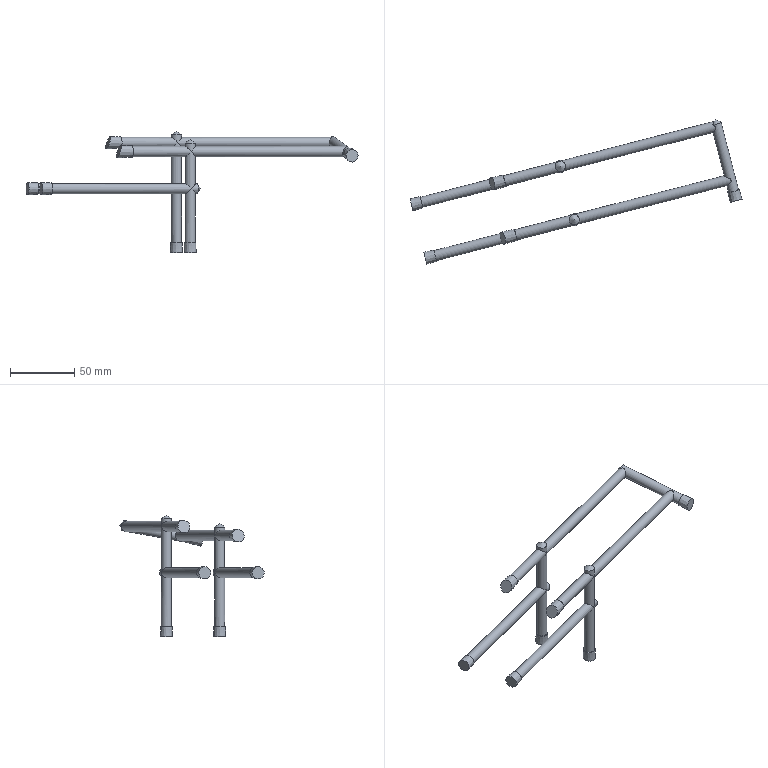Part | STEP file | 车灯-后视镜_id398_x_t | 1 solid | 43 faces | box 259.149 x 112.453 x 94.778 mm | volume 42702 mm3 | cylinder 15 | plane 14 | cone 14 | commonest cylinder face diameters 8 x15
STEP:
#1=CARTESIAN_POINT('',(-127.487,12.001,14.714));
#2=VERTEX_POINT('',#1);
#3=CARTESIAN_POINT('',(-129.485,19.747,14.714));
#4=VERTEX_POINT('',#3);
#5=CARTESIAN_POINT('',(-128.486,15.874,14.714));
#6=DIRECTION('',(-0.6847,-0.1766,-0.7071));
#7=DIRECTION('',(-0.6847,-0.1766,0.7071));
#8=AXIS2_PLACEMENT_3D('',#5,#6,#7);
#9=ELLIPSE('',#8,5.657,4.);
#10=EDGE_CURVE('',#2,#4,#9,.T.);
#11=ORIENTED_EDGE('',*,*,#10,.F.);
#12=CARTESIAN_POINT('',(-128.486,15.874,14.714));
#13=DIRECTION('',(0.6847,0.1766,-0.7071));
#14=DIRECTION('',(0.6847,0.1766,0.7071));
#15=AXIS2_PLACEMENT_3D('',#12,#13,#14);
#16=ELLIPSE('',#15,5.657,4.);
#17=EDGE_CURVE('',#4,#2,#16,.T.);
#18=ORIENTED_EDGE('',*,*,#17,.F.);
#19=EDGE_LOOP('',(#11,#18));
#20=FACE_BOUND('',#19,.T.);
#21=CARTESIAN_POINT('',(-127.487,12.001,43.714));
#22=VERTEX_POINT('',#21);
#23=CARTESIAN_POINT('',(-129.485,19.747,43.714));
#24=VERTEX_POINT('',#23);
#25=CARTESIAN_POINT('',(-128.486,15.874,43.714));
#26=DIRECTION('',(0.6847,0.1766,-0.7071));
#27=DIRECTION('',(0.6847,0.1766,0.7071));
#28=AXIS2_PLACEMENT_3D('',#25,#26,#27);
#29=ELLIPSE('',#28,5.657,4.);
#30=EDGE_CURVE('',#22,#24,#29,.T.);
#31=ORIENTED_EDGE('',*,*,#30,.T.);
#32=CARTESIAN_POINT('',(-128.486,15.874,43.714));
#33=DIRECTION('',(-0.6847,-0.1766,-0.7071));
#34=DIRECTION('',(0.6847,0.1766,-0.7071));
#35=AXIS2_PLACEMENT_3D('',#32,#33,#34);
#36=ELLIPSE('',#35,5.657,4.);
#37=EDGE_CURVE('',#24,#22,#36,.T.);
#38=ORIENTED_EDGE('',*,*,#37,.T.);
#39=EDGE_LOOP('',(#31,#38));
#40=FACE_BOUND('',#39,.T.);
#41=CARTESIAN_POINT('',(-128.486,15.874,-34.206));
#42=DIRECTION('',(0.,0.,1.));
#43=DIRECTION('',(-0.9683,-0.2497,0.));
#44=AXIS2_PLACEMENT_3D('',#41,#42,#43);
#45=CYLINDRICAL_SURFACE('',#44,4.);
#46=ADVANCED_FACE('',(#20,#40),#45,.T.);
#47=ORIENTED_EDGE('',*,*,#37,.F.);
#48=CARTESIAN_POINT('',(-128.486,15.874,43.714));
#49=DIRECTION('',(-0.6847,-0.1766,0.7071));
#50=DIRECTION('',(0.6847,0.1766,0.7071));
#51=AXIS2_PLACEMENT_3D('',#48,#49,#50);
#52=ELLIPSE('',#51,5.657,4.);
#53=EDGE_CURVE('',#22,#24,#52,.T.);
#54=ORIENTED_EDGE('',*,*,#53,.F.);
#55=EDGE_LOOP('',(#47,#54));
#56=FACE_BOUND('',#55,.T.);
#57=CARTESIAN_POINT('',(-6.607,48.159,47.628));
#58=VERTEX_POINT('',#57);
#59=CARTESIAN_POINT('',(-5.871,45.306,47.108));
#60=VERTEX_POINT('',#59);
#61=CARTESIAN_POINT('',(-6.4,47.356,43.714));
#62=DIRECTION('',(0.9683,0.2497,0.));
#63=DIRECTION('',(0.,0.,-1.));
#64=AXIS2_PLACEMENT_3D('',#61,#62,#63);
#65=CIRCLE('',#64,4.);
#66=EDGE_CURVE('',#58,#60,#65,.T.);
#67=ORIENTED_EDGE('',*,*,#66,.F.);
#68=CARTESIAN_POINT('',(-6.607,48.159,47.628));
#69=CARTESIAN_POINT('',(-7.16,48.016,47.628));
#70=CARTESIAN_POINT('',(-7.723,48.193,47.564));
#71=CARTESIAN_POINT('',(-8.745,48.599,47.309));
#72=CARTESIAN_POINT('',(-9.21,48.843,47.121));
#73=CARTESIAN_POINT('',(-10.495,49.569,46.31));
#74=CARTESIAN_POINT('',(-11.18,50.053,45.377));
#75=CARTESIAN_POINT('',(-11.339,50.334,43.164));
#76=CARTESIAN_POINT('',(-10.794,50.106,42.047));
#77=CARTESIAN_POINT('',(-9.74,49.476,40.904));
#78=CARTESIAN_POINT('',(-9.342,49.219,40.587));
#79=CARTESIAN_POINT('',(-8.57,48.586,40.078));
#80=CARTESIAN_POINT('',(-8.159,48.193,39.872));
#81=CARTESIAN_POINT('',(-7.882,47.108,39.676));
#82=CARTESIAN_POINT('',(-8.042,46.529,39.705));
#83=CARTESIAN_POINT('',(-8.382,45.48,39.909));
#84=CARTESIAN_POINT('',(-8.581,44.986,40.086));
#85=CARTESIAN_POINT('',(-9.117,43.59,40.865));
#86=CARTESIAN_POINT('',(-9.391,42.791,41.774));
#87=CARTESIAN_POINT('',(-9.197,42.352,43.97));
#88=CARTESIAN_POINT('',(-8.744,42.76,45.063));
#89=CARTESIAN_POINT('',(-7.887,43.686,46.177));
#90=CARTESIAN_POINT('',(-7.573,44.046,46.479));
#91=CARTESIAN_POINT('',(-6.845,44.772,46.94));
#92=CARTESIAN_POINT('',(-6.422,45.164,47.108));
#93=CARTESIAN_POINT('',(-5.871,45.306,47.108));
#94=B_SPLINE_CURVE_WITH_KNOTS('',3,(#68,#69,#70,#71,#72,#73,#74,#75,#76,#77,#78,#79,#80,#81,#82,#83,#84,#85,#86,#87,#88,#89,#90,#91,#92,#93),.UNSPECIFIED.,.F.,.F.,(4,2,2,2,2,2,2,2,2,2,2,2,4),(0.,0.0625,0.125,0.25,0.375,0.4375,0.5,0.5625,0.625,0.75,0.875,0.9375,1.),.UNSPECIFIED.);
#95=EDGE_CURVE('',#58,#60,#94,.T.);
#96=ORIENTED_EDGE('',*,*,#95,.T.);
#97=EDGE_LOOP('',(#67,#96));
#98=FACE_BOUND('',#97,.T.);
#99=CARTESIAN_POINT('',(-127.44,16.144,43.714));
#100=DIRECTION('',(0.9683,0.2497,0.));
#101=DIRECTION('',(0.,0.,1.));
#102=AXIS2_PLACEMENT_3D('',#99,#100,#101);
#103=CYLINDRICAL_SURFACE('',#102,4.);
#104=ADVANCED_FACE('',(#56,#98),#103,.T.);
#105=CARTESIAN_POINT('',(-138.224,53.639,14.714));
#106=VERTEX_POINT('',#105);
#107=CARTESIAN_POINT('',(-140.222,61.385,14.714));
#108=VERTEX_POINT('',#107);
#109=CARTESIAN_POINT('',(-139.223,57.512,14.714));
#110=DIRECTION('',(-0.6847,-0.1766,-0.7071));
#111=DIRECTION('',(-0.6847,-0.1766,0.7071));
#112=AXIS2_PLACEMENT_3D('',#109,#110,#111);
#113=ELLIPSE('',#112,5.657,4.);
#114=EDGE_CURVE('',#106,#108,#113,.T.);
#115=ORIENTED_EDGE('',*,*,#114,.F.);
#116=CARTESIAN_POINT('',(-139.223,57.512,14.714));
#117=DIRECTION('',(0.6847,0.1766,-0.7071));
#118=DIRECTION('',(0.6847,0.1766,0.7071));
#119=AXIS2_PLACEMENT_3D('',#116,#117,#118);
#120=ELLIPSE('',#119,5.657,4.);
#121=EDGE_CURVE('',#108,#106,#120,.T.);
#122=ORIENTED_EDGE('',*,*,#121,.F.);
#123=EDGE_LOOP('',(#115,#122));
#124=FACE_BOUND('',#123,.T.);
#125=CARTESIAN_POINT('',(-138.224,53.639,50.714));
#126=VERTEX_POINT('',#125);
#127=CARTESIAN_POINT('',(-140.222,61.385,50.714));
#128=VERTEX_POINT('',#127);
#129=CARTESIAN_POINT('',(-139.223,57.512,50.714));
#130=DIRECTION('',(0.6847,0.1766,-0.7071));
#131=DIRECTION('',(0.6847,0.1766,0.7071));
#132=AXIS2_PLACEMENT_3D('',#129,#130,#131);
#133=ELLIPSE('',#132,5.657,4.);
#134=EDGE_CURVE('',#126,#128,#133,.T.);
#135=ORIENTED_EDGE('',*,*,#134,.T.);
#136=CARTESIAN_POINT('',(-139.223,57.512,50.714));
#137=DIRECTION('',(-0.6847,-0.1766,-0.7071));
#138=DIRECTION('',(0.6847,0.1766,-0.7071));
#139=AXIS2_PLACEMENT_3D('',#136,#137,#138);
#140=ELLIPSE('',#139,5.657,4.);
#141=EDGE_CURVE('',#128,#126,#140,.T.);
#142=ORIENTED_EDGE('',*,*,#141,.T.);
#143=EDGE_LOOP('',(#135,#142));
#144=FACE_BOUND('',#143,.T.);
#145=CARTESIAN_POINT('',(-139.223,57.512,-34.206));
#146=DIRECTION('',(0.,0.,1.));
#147=DIRECTION('',(-0.9683,-0.2497,0.));
#148=AXIS2_PLACEMENT_3D('',#145,#146,#147);
#149=CYLINDRICAL_SURFACE('',#148,4.);
#150=ADVANCED_FACE('',(#124,#144),#149,.T.);
#151=ORIENTED_EDGE('',*,*,#141,.F.);
#152=CARTESIAN_POINT('',(-139.223,57.512,50.714));
#153=DIRECTION('',(-0.6847,-0.1766,0.7071));
#154=DIRECTION('',(0.6847,0.1766,0.7071));
#155=AXIS2_PLACEMENT_3D('',#152,#153,#154);
#156=ELLIPSE('',#155,5.657,4.);
#157=EDGE_CURVE('',#126,#128,#156,.T.);
#158=ORIENTED_EDGE('',*,*,#157,.F.);
#159=EDGE_LOOP('',(#151,#158));
#160=FACE_BOUND('',#159,.T.);
#161=CARTESIAN_POINT('',(-20.16,89.995,54.324));
#162=VERTEX_POINT('',#161);
#163=CARTESIAN_POINT('',(-19.657,91.292,47.913));
#164=VERTEX_POINT('',#163);
#165=CARTESIAN_POINT('',(-20.16,89.995,54.324));
#166=CARTESIAN_POINT('',(-19.714,90.574,54.109));
#167=CARTESIAN_POINT('',(-19.345,91.232,53.745));
#168=CARTESIAN_POINT('',(-19.474,92.149,52.54));
#169=CARTESIAN_POINT('',(-19.692,92.385,51.788));
#170=CARTESIAN_POINT('',(-19.388,92.561,50.693));
#171=CARTESIAN_POINT('',(-19.212,92.586,50.351));
#172=CARTESIAN_POINT('',(-18.883,92.587,49.883));
#173=CARTESIAN_POINT('',(-18.763,92.583,49.735));
#174=CARTESIAN_POINT('',(-18.513,92.56,49.448));
#175=CARTESIAN_POINT('',(-18.354,92.556,49.319));
#176=CARTESIAN_POINT('',(-18.221,92.441,48.978));
#177=CARTESIAN_POINT('',(-18.386,92.324,48.842));
#178=CARTESIAN_POINT('',(-18.622,92.131,48.617));
#179=CARTESIAN_POINT('',(-18.748,92.031,48.516));
#180=CARTESIAN_POINT('',(-19.13,91.726,48.229));
#181=CARTESIAN_POINT('',(-19.391,91.513,48.063));
#182=CARTESIAN_POINT('',(-19.657,91.292,47.913));
#183=B_SPLINE_CURVE_WITH_KNOTS('',3,(#165,#166,#167,#168,#169,#170,#171,#172,#173,#174,#175,#176,#177,#178,#179,#180,#181,#182),.UNSPECIFIED.,.F.,.F.,(4,2,2,2,2,2,2,2,4),(0.,0.25,0.5,0.625,0.6875,0.75,0.8125,0.875,1.),.UNSPECIFIED.);
#184=EDGE_CURVE('',#162,#164,#183,.T.);
#185=ORIENTED_EDGE('',*,*,#184,.T.);
#186=CARTESIAN_POINT('',(-17.661,91.028,47.311));
#187=VERTEX_POINT('',#186);
#188=CARTESIAN_POINT('',(-19.657,91.292,47.913));
#189=CARTESIAN_POINT('',(-19.38,91.203,47.754));
#190=CARTESIAN_POINT('',(-19.088,91.112,47.618));
#191=CARTESIAN_POINT('',(-18.781,91.047,47.514));
#192=CARTESIAN_POINT('',(-18.553,90.999,47.436));
#193=CARTESIAN_POINT('',(-18.313,90.965,47.374));
#194=CARTESIAN_POINT('',(-18.07,90.972,47.34));
#195=CARTESIAN_POINT('',(-17.933,90.976,47.321));
#196=CARTESIAN_POINT('',(-17.795,90.994,47.311));
#197=CARTESIAN_POINT('',(-17.661,91.028,47.311));
#198=B_SPLINE_CURVE_WITH_KNOTS('',3,(#188,#189,#190,#191,#192,#193,#194,#195,#196,#197),.UNSPECIFIED.,.F.,.F.,(4,3,3,4),(0.,0.4633,0.8077,1.),.UNSPECIFIED.);
#199=EDGE_CURVE('',#164,#187,#198,.T.);
#200=ORIENTED_EDGE('',*,*,#199,.T.);
#201=CARTESIAN_POINT('',(-16.935,88.21,46.797));
#202=VERTEX_POINT('',#201);
#203=CARTESIAN_POINT('',(-17.137,88.994,50.714));
#204=DIRECTION('',(0.9683,0.2497,0.));
#205=DIRECTION('',(0.,0.,-1.));
#206=AXIS2_PLACEMENT_3D('',#203,#204,#205);
#207=CIRCLE('',#206,4.);
#208=EDGE_CURVE('',#202,#187,#207,.T.);
#209=ORIENTED_EDGE('',*,*,#208,.F.);
#210=CARTESIAN_POINT('',(-16.935,88.21,46.797));
#211=CARTESIAN_POINT('',(-17.603,88.037,46.797));
#212=CARTESIAN_POINT('',(-18.061,87.463,46.889));
#213=CARTESIAN_POINT('',(-18.841,86.422,47.26));
#214=CARTESIAN_POINT('',(-19.169,85.887,47.543));
#215=CARTESIAN_POINT('',(-19.702,84.946,48.355));
#216=CARTESIAN_POINT('',(-19.903,84.537,48.896));
#217=CARTESIAN_POINT('',(-20.06,84.089,50.174));
#218=CARTESIAN_POINT('',(-20.006,84.072,50.884));
#219=CARTESIAN_POINT('',(-19.551,84.601,52.81));
#220=CARTESIAN_POINT('',(-18.875,85.556,53.721));
#221=CARTESIAN_POINT('',(-18.394,87.047,54.405));
#222=CARTESIAN_POINT('',(-18.322,87.369,54.52));
#223=CARTESIAN_POINT('',(-18.38,88.026,54.679));
#224=CARTESIAN_POINT('',(-18.529,88.349,54.717));
#225=CARTESIAN_POINT('',(-19.136,89.165,54.708));
#226=CARTESIAN_POINT('',(-19.673,89.587,54.571));
#227=CARTESIAN_POINT('',(-20.16,89.995,54.324));
#228=B_SPLINE_CURVE_WITH_KNOTS('',3,(#210,#211,#212,#213,#214,#215,#216,#217,#218,#219,#220,#221,#222,#223,#224,#225,#226,#227),.UNSPECIFIED.,.F.,.F.,(4,2,2,2,2,2,2,2,4),(0.,0.125,0.25,0.375,0.5,0.75,0.8125,0.875,1.),.UNSPECIFIED.);
#229=EDGE_CURVE('',#202,#162,#228,.T.);
#230=ORIENTED_EDGE('',*,*,#229,.T.);
#231=EDGE_LOOP('',(#185,#200,#209,#230));
#232=FACE_BOUND('',#231,.T.);
#233=CARTESIAN_POINT('',(-138.177,57.782,50.714));
#234=DIRECTION('',(0.9683,0.2497,0.));
#235=DIRECTION('',(0.,0.,1.));
#236=AXIS2_PLACEMENT_3D('',#233,#234,#235);
#237=CYLINDRICAL_SURFACE('',#236,4.);
#238=ADVANCED_FACE('',(#160,#232),#237,.T.);
#239=CARTESIAN_POINT('',(-8.025,37.639,41.832));
#240=VERTEX_POINT('',#239);
#241=CARTESIAN_POINT('',(-4.152,38.638,41.832));
#242=DIRECTION('',(0.2459,-0.9536,-0.1736));
#243=DIRECTION('',(-0.9683,-0.2497,0.));
#244=AXIS2_PLACEMENT_3D('',#241,#242,#243);
#245=CIRCLE('',#244,4.);
#246=EDGE_CURVE('',#240,#240,#245,.T.);
#247=ORIENTED_EDGE('',*,*,#246,.T.);
#248=EDGE_LOOP('',(#247));
#249=FACE_BOUND('',#248,.T.);
#250=CARTESIAN_POINT('',(-4.348,39.401,37.366));
#251=VERTEX_POINT('',#250);
#252=CARTESIAN_POINT('',(-4.152,38.638,41.832));
#253=DIRECTION('',(-0.2459,0.9536,0.1736));
#254=DIRECTION('',(-0.04336,0.1681,-0.9848));
#255=AXIS2_PLACEMENT_3D('',#252,#253,#254);
#256=CIRCLE('',#255,4.535);
#257=EDGE_CURVE('',#251,#251,#256,.T.);
#258=ORIENTED_EDGE('',*,*,#257,.T.);
#259=EDGE_LOOP('',(#258));
#260=FACE_BOUND('',#259,.T.);
#261=CARTESIAN_POINT('',(-4.152,38.638,41.832));
#262=DIRECTION('',(-0.2459,0.9536,0.1736));
#263=DIRECTION('',(0.04336,-0.1681,0.9848));
#264=AXIS2_PLACEMENT_3D('',#261,#262,#263);
#265=PLANE('',#264);
#266=ADVANCED_FACE('',(#249,#260),#265,.T.);
#267=CARTESIAN_POINT('',(-2.104,30.689,35.497));
#268=VERTEX_POINT('',#267);
#269=CARTESIAN_POINT('',(-2.102,30.69,40.359));
#270=DIRECTION('',(0.2498,-0.9683,0.));
#271=DIRECTION('',(-0.0003877,-0.0001,-1.));
#272=AXIS2_PLACEMENT_3D('',#269,#270,#271);
#273=ELLIPSE('',#272,4.862,4.788);
#274=EDGE_CURVE('',#268,#268,#273,.T.);
#275=ORIENTED_EDGE('',*,*,#274,.F.);
#276=EDGE_LOOP('',(#275));
#277=FACE_BOUND('',#276,.T.);
#278=ORIENTED_EDGE('',*,*,#257,.F.);
#279=EDGE_LOOP('',(#278));
#280=FACE_BOUND('',#279,.T.);
#281=CARTESIAN_POINT('',(-4.152,38.638,41.832));
#282=DIRECTION('',(0.2459,-0.9536,-0.1736));
#283=DIRECTION('',(-0.04336,0.1681,-0.9848));
#284=AXIS2_PLACEMENT_3D('',#281,#282,#283);
#285=CONICAL_SURFACE('',#284,4.535,1.738);
#286=ADVANCED_FACE('',(#277,#280),#285,.T.);
#287=ORIENTED_EDGE('',*,*,#95,.F.);
#288=CARTESIAN_POINT('',(-5.871,45.306,47.108));
#289=CARTESIAN_POINT('',(-5.873,46.298,47.278));
#290=CARTESIAN_POINT('',(-6.124,47.281,47.456));
#291=CARTESIAN_POINT('',(-6.607,48.159,47.628));
#292=B_SPLINE_CURVE_WITH_KNOTS('',3,(#288,#289,#290,#291),.UNSPECIFIED.,.F.,.F.,(4,4),(0.,1.),.UNSPECIFIED.);
#293=EDGE_CURVE('',#60,#58,#292,.T.);
#294=ORIENTED_EDGE('',*,*,#293,.F.);
#295=EDGE_LOOP('',(#287,#294));
#296=FACE_BOUND('',#295,.T.);
#297=ORIENTED_EDGE('',*,*,#199,.F.);
#298=CARTESIAN_POINT('',(-17.696,91.163,51.397));
#299=DIRECTION('',(-0.2459,0.9536,0.1736));
#300=DIRECTION('',(0.9683,0.2497,0.));
#301=AXIS2_PLACEMENT_3D('',#298,#299,#300);
#302=CIRCLE('',#301,4.);
#303=EDGE_CURVE('',#162,#164,#302,.T.);
#304=ORIENTED_EDGE('',*,*,#303,.F.);
#305=ORIENTED_EDGE('',*,*,#229,.F.);
#306=CARTESIAN_POINT('',(-17.661,91.028,47.311));
#307=CARTESIAN_POINT('',(-17.193,90.171,47.144));
#308=CARTESIAN_POINT('',(-16.939,89.193,46.965));
#309=CARTESIAN_POINT('',(-16.935,88.21,46.797));
#310=B_SPLINE_CURVE_WITH_KNOTS('',3,(#306,#307,#308,#309),.UNSPECIFIED.,.F.,.F.,(4,4),(0.,1.),.UNSPECIFIED.);
#311=EDGE_CURVE('',#187,#202,#310,.T.);
#312=ORIENTED_EDGE('',*,*,#311,.F.);
#313=EDGE_LOOP('',(#297,#304,#305,#312));
#314=FACE_BOUND('',#313,.T.);
#315=ORIENTED_EDGE('',*,*,#246,.F.);
#316=EDGE_LOOP('',(#315));
#317=FACE_BOUND('',#316,.T.);
#318=CARTESIAN_POINT('',(15.993,-39.482,27.607));
#319=DIRECTION('',(-0.2459,0.9536,0.1736));
#320=DIRECTION('',(0.04336,-0.1681,0.9848));
#321=AXIS2_PLACEMENT_3D('',#318,#319,#320);
#322=CYLINDRICAL_SURFACE('',#321,4.);
#323=ADVANCED_FACE('',(#296,#314,#317),#322,.T.);
#324=ORIENTED_EDGE('',*,*,#184,.F.);
#325=ORIENTED_EDGE('',*,*,#303,.T.);
#326=EDGE_LOOP('',(#324,#325));
#327=FACE_BOUND('',#326,.T.);
#328=CARTESIAN_POINT('',(-18.36,93.736,51.865));
#329=VERTEX_POINT('',#328);
#330=VERTEX_LOOP('',#329);
#331=FACE_BOUND('',#330,.T.);
#332=CARTESIAN_POINT('',(-18.36,93.736,51.865));
#333=DIRECTION('',(0.2459,-0.9536,-0.1736));
#334=DIRECTION('',(0.04336,-0.1681,0.9848));
#335=AXIS2_PLACEMENT_3D('',#332,#333,#334);
#336=CONICAL_SURFACE('',#335,0.,56.);
#337=ADVANCED_FACE('',(#327,#331),#336,.T.);
#338=ORIENTED_EDGE('',*,*,#274,.T.);
#339=EDGE_LOOP('',(#338));
#340=FACE_OUTER_BOUND('',#339,.T.);
#341=CARTESIAN_POINT('',(-10.125,28.621,33.596));
#342=DIRECTION('',(-0.2498,0.9683,0.));
#343=DIRECTION('',(-0.9683,-0.2498,0.));
#344=AXIS2_PLACEMENT_3D('',#341,#342,#343);
#345=PLANE('',#344);
#346=ADVANCED_FACE('',(#340),#345,.F.);
#347=ORIENTED_EDGE('',*,*,#208,.T.);
#348=ORIENTED_EDGE('',*,*,#311,.T.);
#349=EDGE_LOOP('',(#347,#348));
#350=FACE_OUTER_BOUND('',#349,.T.);
#351=CARTESIAN_POINT('',(-14.524,89.668,50.714));
#352=DIRECTION('',(-0.9683,-0.2497,0.));
#353=DIRECTION('',(0.,0.,1.));
#354=AXIS2_PLACEMENT_3D('',#351,#352,#353);
#355=CONICAL_SURFACE('',#354,0.,56.);
#356=ADVANCED_FACE('',(#350),#355,.T.);
#357=CARTESIAN_POINT('',(-143.223,57.512,56.794));
#358=VERTEX_POINT('',#357);
#359=CARTESIAN_POINT('',(-139.223,57.512,56.794));
#360=DIRECTION('',(0.,0.,1.));
#361=DIRECTION('',(-1.,0.,0.));
#362=AXIS2_PLACEMENT_3D('',#359,#360,#361);
#363=CIRCLE('',#362,4.);
#364=EDGE_CURVE('',#358,#358,#363,.T.);
#365=ORIENTED_EDGE('',*,*,#364,.T.);
#366=EDGE_LOOP('',(#365));
#367=FACE_BOUND('',#366,.T.);
#368=CARTESIAN_POINT('',(-139.223,57.512,59.492));
#369=VERTEX_POINT('',#368);
#370=VERTEX_LOOP('',#369);
#371=FACE_BOUND('',#370,.T.);
#372=CARTESIAN_POINT('',(-139.223,57.512,59.492));
#373=DIRECTION('',(0.,0.,-1.));
#374=DIRECTION('',(-0.9683,-0.2497,0.));
#375=AXIS2_PLACEMENT_3D('',#372,#373,#374);
#376=CONICAL_SURFACE('',#375,0.,56.);
#377=ADVANCED_FACE('',(#367,#371),#376,.T.);
#378=ORIENTED_EDGE('',*,*,#364,.F.);
#379=EDGE_LOOP('',(#378));
#380=FACE_BOUND('',#379,.T.);
#381=ORIENTED_EDGE('',*,*,#157,.T.);
#382=CARTESIAN_POINT('',(-139.223,57.512,50.714));
#383=DIRECTION('',(0.6847,0.1766,0.7071));
#384=DIRECTION('',(0.6847,0.1766,-0.7071));
#385=AXIS2_PLACEMENT_3D('',#382,#383,#384);
#386=ELLIPSE('',#385,5.657,4.);
#387=EDGE_CURVE('',#128,#126,#386,.T.);
#388=ORIENTED_EDGE('',*,*,#387,.T.);
#389=EDGE_LOOP('',(#381,#388));
#390=FACE_BOUND('',#389,.T.);
#391=CARTESIAN_POINT('',(-139.223,57.512,-34.206));
#392=DIRECTION('',(0.,0.,1.));
#393=DIRECTION('',(-0.9683,-0.2497,0.));
#394=AXIS2_PLACEMENT_3D('',#391,#392,#393);
#395=CYLINDRICAL_SURFACE('',#394,4.);
#396=ADVANCED_FACE('',(#380,#390),#395,.T.);
#397=CARTESIAN_POINT('',(-194.112,43.358,45.825));
#398=VERTEX_POINT('',#397);
#399=CARTESIAN_POINT('',(-192.407,43.797,50.661));
#400=DIRECTION('',(-0.9099,-0.2346,0.342));
#401=DIRECTION('',(-0.3312,-0.0854,-0.9397));
#402=AXIS2_PLACEMENT_3D('',#399,#400,#401);
#403=ELLIPSE('',#402,5.147,4.836);
#404=EDGE_CURVE('',#398,#398,#403,.T.);
#405=ORIENTED_EDGE('',*,*,#404,.T.);
#406=EDGE_LOOP('',(#405));
#407=FACE_OUTER_BOUND('',#406,.T.);
#408=CARTESIAN_POINT('',(-192.52,23.906,36.714));
#409=DIRECTION('',(-0.9099,-0.2346,0.342));
#410=DIRECTION('',(0.3518,0.,0.9361));
#411=AXIS2_PLACEMENT_3D('',#408,#409,#410);
#412=PLANE('',#411);
#413=ADVANCED_FACE('',(#407),#412,.T.);
#414=ORIENTED_EDGE('',*,*,#404,.F.);
#415=EDGE_LOOP('',(#414));
#416=FACE_BOUND('',#415,.T.);
#417=CARTESIAN_POINT('',(-182.798,46.275,46.179));
#418=VERTEX_POINT('',#417);
#419=CARTESIAN_POINT('',(-182.798,46.275,50.714));
#420=DIRECTION('',(0.9683,0.2497,0.));
#421=DIRECTION('',(0.,0.,-1.));
#422=AXIS2_PLACEMENT_3D('',#419,#420,#421);
#423=CIRCLE('',#422,4.535);
#424=EDGE_CURVE('',#418,#418,#423,.T.);
#425=ORIENTED_EDGE('',*,*,#424,.F.);
#426=EDGE_LOOP('',(#425));
#427=FACE_BOUND('',#426,.T.);
#428=CARTESIAN_POINT('',(-182.798,46.275,50.714));
#429=DIRECTION('',(-0.9683,-0.2497,0.));
#430=DIRECTION('',(0.,0.,-1.));
#431=AXIS2_PLACEMENT_3D('',#428,#429,#430);
#432=CONICAL_SURFACE('',#431,4.535,1.738);
#433=ADVANCED_FACE('',(#416,#427),#432,.T.);
#434=CARTESIAN_POINT('',(-183.796,50.149,50.714));
#435=VERTEX_POINT('',#434);
#436=CARTESIAN_POINT('',(-182.798,46.275,50.714));
#437=DIRECTION('',(-0.9683,-0.2497,0.));
#438=DIRECTION('',(-0.2497,0.9683,0.));
#439=AXIS2_PLACEMENT_3D('',#436,#437,#438);
#440=CIRCLE('',#439,4.);
#441=EDGE_CURVE('',#435,#435,#440,.T.);
#442=ORIENTED_EDGE('',*,*,#441,.T.);
#443=EDGE_LOOP('',(#442));
#444=FACE_BOUND('',#443,.T.);
#445=ORIENTED_EDGE('',*,*,#424,.T.);
#446=EDGE_LOOP('',(#445));
#447=FACE_BOUND('',#446,.T.);
#448=CARTESIAN_POINT('',(-182.798,46.275,50.714));
#449=DIRECTION('',(0.9683,0.2497,0.));
#450=DIRECTION('',(0.,0.,1.));
#451=AXIS2_PLACEMENT_3D('',#448,#449,#450);
#452=PLANE('',#451);
#453=ADVANCED_FACE('',(#444,#447),#452,.T.);
#454=ORIENTED_EDGE('',*,*,#387,.F.);
#455=ORIENTED_EDGE('',*,*,#134,.F.);
#456=EDGE_LOOP('',(#454,#455));
#457=FACE_BOUND('',#456,.T.);
#458=ORIENTED_EDGE('',*,*,#441,.F.);
#459=EDGE_LOOP('',(#458));
#460=FACE_BOUND('',#459,.T.);
#461=CARTESIAN_POINT('',(-138.177,57.782,50.714));
#462=DIRECTION('',(0.9683,0.2497,0.));
#463=DIRECTION('',(0.,0.,1.));
#464=AXIS2_PLACEMENT_3D('',#461,#462,#463);
#465=CYLINDRICAL_SURFACE('',#464,4.);
#466=ADVANCED_FACE('',(#457,#460),#465,.T.);
#467=CARTESIAN_POINT('',(-134.069,59.872,18.588));
#468=VERTEX_POINT('',#467);
#469=CARTESIAN_POINT('',(-133.82,58.905,14.714));
#470=DIRECTION('',(0.9683,0.2497,0.));
#471=DIRECTION('',(-0.06235,0.2418,0.9683));
#472=AXIS2_PLACEMENT_3D('',#469,#470,#471);
#473=CIRCLE('',#472,4.);
#474=EDGE_CURVE('',#468,#468,#473,.T.);
#475=ORIENTED_EDGE('',*,*,#474,.T.);
#476=EDGE_LOOP('',(#475));
#477=FACE_BOUND('',#476,.T.);
#478=CARTESIAN_POINT('',(-131.207,59.579,14.714));
#479=VERTEX_POINT('',#478);
#480=VERTEX_LOOP('',#479);
#481=FACE_BOUND('',#480,.T.);
#482=CARTESIAN_POINT('',(-131.207,59.579,14.714));
#483=DIRECTION('',(-0.9683,-0.2497,0.));
#484=DIRECTION('',(0.,0.,1.));
#485=AXIS2_PLACEMENT_3D('',#482,#483,#484);
#486=CONICAL_SURFACE('',#485,0.,56.);
#487=ADVANCED_FACE('',(#477,#481),#486,.T.);
#488=ORIENTED_EDGE('',*,*,#474,.F.);
#489=EDGE_LOOP('',(#488));
#490=FACE_BOUND('',#489,.T.);
#491=ORIENTED_EDGE('',*,*,#121,.T.);
#492=CARTESIAN_POINT('',(-139.223,57.512,14.714));
#493=DIRECTION('',(0.6847,0.1766,0.7071));
#494=DIRECTION('',(-0.6847,-0.1766,0.7071));
#495=AXIS2_PLACEMENT_3D('',#492,#493,#494);
#496=ELLIPSE('',#495,5.657,4.);
#497=EDGE_CURVE('',#106,#108,#496,.T.);
#498=ORIENTED_EDGE('',*,*,#497,.T.);
#499=EDGE_LOOP('',(#491,#498));
#500=FACE_BOUND('',#499,.T.);
#501=CARTESIAN_POINT('',(-215.643,37.806,14.714));
#502=DIRECTION('',(0.9683,0.2497,0.));
#503=DIRECTION('',(0.,0.,1.));
#504=AXIS2_PLACEMENT_3D('',#501,#502,#503);
#505=CYLINDRICAL_SURFACE('',#504,4.);
#506=ADVANCED_FACE('',(#490,#500),#505,.T.);
#507=CARTESIAN_POINT('',(-248.674,33.419,14.714));
#508=VERTEX_POINT('',#507);
#509=CARTESIAN_POINT('',(-247.675,29.546,14.714));
#510=DIRECTION('',(-0.9683,-0.2497,0.));
#511=DIRECTION('',(-0.2497,0.9683,0.));
#512=AXIS2_PLACEMENT_3D('',#509,#510,#511);
#513=CIRCLE('',#512,4.);
#514=EDGE_CURVE('',#508,#508,#513,.T.);
#515=ORIENTED_EDGE('',*,*,#514,.T.);
#516=EDGE_LOOP('',(#515));
#517=FACE_BOUND('',#516,.T.);
#518=CARTESIAN_POINT('',(-247.675,29.546,10.179));
#519=VERTEX_POINT('',#518);
#520=CARTESIAN_POINT('',(-247.675,29.546,14.714));
#521=DIRECTION('',(0.9683,0.2497,0.));
#522=DIRECTION('',(0.,0.,-1.));
#523=AXIS2_PLACEMENT_3D('',#520,#521,#522);
#524=CIRCLE('',#523,4.535);
#525=EDGE_CURVE('',#519,#519,#524,.T.);
#526=ORIENTED_EDGE('',*,*,#525,.T.);
#527=EDGE_LOOP('',(#526));
#528=FACE_BOUND('',#527,.T.);
#529=CARTESIAN_POINT('',(-247.675,29.546,14.714));
#530=DIRECTION('',(0.9683,0.2497,0.));
#531=DIRECTION('',(0.,0.,1.));
#532=AXIS2_PLACEMENT_3D('',#529,#530,#531);
#533=PLANE('',#532);
#534=ADVANCED_FACE('',(#517,#528),#533,.T.);
#535=CARTESIAN_POINT('',(-255.124,26.393,10.088));
#536=VERTEX_POINT('',#535);
#537=CARTESIAN_POINT('',(-255.422,27.548,14.714));
#538=DIRECTION('',(-0.9683,-0.2497,0.));
#539=DIRECTION('',(0.06235,-0.2418,-0.9683));
#540=AXIS2_PLACEMENT_3D('',#537,#538,#539);
#541=CIRCLE('',#540,4.778);
#542=EDGE_CURVE('',#536,#536,#541,.T.);
#543=ORIENTED_EDGE('',*,*,#542,.F.);
#544=EDGE_LOOP('',(#543));
#545=FACE_BOUND('',#544,.T.);
#546=ORIENTED_EDGE('',*,*,#525,.F.);
#547=EDGE_LOOP('',(#546));
#548=FACE_BOUND('',#547,.T.);
#549=CARTESIAN_POINT('',(-247.675,29.546,14.714));
#550=DIRECTION('',(-0.9683,-0.2497,0.));
#551=DIRECTION('',(0.,0.,-1.));
#552=AXIS2_PLACEMENT_3D('',#549,#550,#551);
#553=CONICAL_SURFACE('',#552,4.535,1.738);
#554=ADVANCED_FACE('',(#545,#548),#553,.T.);
#555=CARTESIAN_POINT('',(-139.223,57.512,14.714));
#556=DIRECTION('',(-0.6847,-0.1766,0.7071));
#557=DIRECTION('',(0.6847,0.1766,0.7071));
#558=AXIS2_PLACEMENT_3D('',#555,#556,#557);
#559=ELLIPSE('',#558,5.657,4.);
#560=EDGE_CURVE('',#108,#106,#559,.T.);
#561=ORIENTED_EDGE('',*,*,#560,.T.);
#562=ORIENTED_EDGE('',*,*,#114,.T.);
#563=EDGE_LOOP('',(#561,#562));
#564=FACE_BOUND('',#563,.T.);
#565=ORIENTED_EDGE('',*,*,#514,.F.);
#566=EDGE_LOOP('',(#565));
#567=FACE_BOUND('',#566,.T.);
#568=CARTESIAN_POINT('',(-215.643,37.806,14.714));
#569=DIRECTION('',(0.9683,0.2497,0.));
#570=DIRECTION('',(0.,0.,1.));
#571=AXIS2_PLACEMENT_3D('',#568,#569,#570);
#572=CYLINDRICAL_SURFACE('',#571,4.);
#573=ADVANCED_FACE('',(#564,#567),#572,.T.);
#574=ORIENTED_EDGE('',*,*,#542,.T.);
#575=EDGE_LOOP('',(#574));
#576=FACE_OUTER_BOUND('',#575,.T.);
#577=CARTESIAN_POINT('',(-255.422,27.548,14.714));
#578=DIRECTION('',(0.9683,0.2497,0.));
#579=DIRECTION('',(0.,0.,-1.));
#580=AXIS2_PLACEMENT_3D('',#577,#578,#579);
#581=PLANE('',#580);
#582=ADVANCED_FACE('',(#576),#581,.F.);
#583=CARTESIAN_POINT('',(-134.445,57.512,-35.286));
#584=VERTEX_POINT('',#583);
#585=CARTESIAN_POINT('',(-139.223,57.512,-35.286));
#586=DIRECTION('',(0.,0.,-1.));
#587=DIRECTION('',(1.,0.,0.));
#588=AXIS2_PLACEMENT_3D('',#585,#586,#587);
#589=CIRCLE('',#588,4.778);
#590=EDGE_CURVE('',#584,#584,#589,.T.);
#591=ORIENTED_EDGE('',*,*,#590,.T.);
#592=EDGE_LOOP('',(#591));
#593=FACE_OUTER_BOUND('',#592,.T.);
#594=CARTESIAN_POINT('',(-139.223,57.512,-35.286));
#595=DIRECTION('',(0.,0.,1.));
#596=DIRECTION('',(0.9683,0.2497,0.));
#597=AXIS2_PLACEMENT_3D('',#594,#595,#596);
#598=PLANE('',#597);
#599=ADVANCED_FACE('',(#593),#598,.F.);
#600=ORIENTED_EDGE('',*,*,#590,.F.);
#601=EDGE_LOOP('',(#600));
#602=FACE_BOUND('',#601,.T.);
#603=CARTESIAN_POINT('',(-134.832,58.644,-27.286));
#604=VERTEX_POINT('',#603);
#605=CARTESIAN_POINT('',(-139.223,57.512,-27.286));
#606=DIRECTION('',(0.,0.,1.));
#607=DIRECTION('',(0.9683,0.2497,0.));
#608=AXIS2_PLACEMENT_3D('',#605,#606,#607);
#609=CIRCLE('',#608,4.535);
#610=EDGE_CURVE('',#604,#604,#609,.T.);
#611=ORIENTED_EDGE('',*,*,#610,.F.);
#612=EDGE_LOOP('',(#611));
#613=FACE_BOUND('',#612,.T.);
#614=CARTESIAN_POINT('',(-139.223,57.512,-27.286));
#615=DIRECTION('',(0.,0.,-1.));
#616=DIRECTION('',(0.9683,0.2497,0.));
#617=AXIS2_PLACEMENT_3D('',#614,#615,#616);
#618=CONICAL_SURFACE('',#617,4.535,1.738);
#619=ADVANCED_FACE('',(#602,#613),#618,.T.);
#620=CARTESIAN_POINT('',(-143.096,56.513,-27.286));
#621=VERTEX_POINT('',#620);
#622=CARTESIAN_POINT('',(-139.223,57.512,-27.286));
#623=DIRECTION('',(0.,0.,-1.));
#624=DIRECTION('',(-0.9683,-0.2497,0.));
#625=AXIS2_PLACEMENT_3D('',#622,#623,#624);
#626=CIRCLE('',#625,4.);
#627=EDGE_CURVE('',#621,#621,#626,.T.);
#628=ORIENTED_EDGE('',*,*,#627,.T.);
#629=EDGE_LOOP('',(#628));
#630=FACE_BOUND('',#629,.T.);
#631=ORIENTED_EDGE('',*,*,#610,.T.);
#632=EDGE_LOOP('',(#631));
#633=FACE_BOUND('',#632,.T.);
#634=CARTESIAN_POINT('',(-139.223,57.512,-27.286));
#635=DIRECTION('',(0.,0.,1.));
#636=DIRECTION('',(-0.9683,-0.2497,0.));
#637=AXIS2_PLACEMENT_3D('',#634,#635,#636);
#638=PLANE('',#637);
#639=ADVANCED_FACE('',(#630,#633),#638,.T.);
#640=ORIENTED_EDGE('',*,*,#497,.F.);
#641=ORIENTED_EDGE('',*,*,#560,.F.);
#642=EDGE_LOOP('',(#640,#641));
#643=FACE_BOUND('',#642,.T.);
#644=ORIENTED_EDGE('',*,*,#627,.F.);
#645=EDGE_LOOP('',(#644));
#646=FACE_BOUND('',#645,.T.);
#647=CARTESIAN_POINT('',(-139.223,57.512,-34.206));
#648=DIRECTION('',(0.,0.,1.));
#649=DIRECTION('',(-0.9683,-0.2497,0.));
#650=AXIS2_PLACEMENT_3D('',#647,#648,#649);
#651=CYLINDRICAL_SURFACE('',#650,4.);
#652=ADVANCED_FACE('',(#643,#646),#651,.T.);
#653=ORIENTED_EDGE('',*,*,#66,.T.);
#654=ORIENTED_EDGE('',*,*,#293,.T.);
#655=EDGE_LOOP('',(#653,#654));
#656=FACE_OUTER_BOUND('',#655,.T.);
#657=CARTESIAN_POINT('',(-3.787,48.03,43.714));
#658=DIRECTION('',(-0.9683,-0.2497,0.));
#659=DIRECTION('',(0.,0.,1.));
#660=AXIS2_PLACEMENT_3D('',#657,#658,#659);
#661=CONICAL_SURFACE('',#660,0.,56.);
#662=ADVANCED_FACE('',(#656),#661,.T.);
#663=CARTESIAN_POINT('',(-132.486,15.874,50.294));
#664=VERTEX_POINT('',#663);
#665=CARTESIAN_POINT('',(-128.486,15.874,50.294));
#666=DIRECTION('',(0.,0.,1.));
#667=DIRECTION('',(-1.,0.,0.));
#668=AXIS2_PLACEMENT_3D('',#665,#666,#667);
#669=CIRCLE('',#668,4.);
#670=EDGE_CURVE('',#664,#664,#669,.T.);
#671=ORIENTED_EDGE('',*,*,#670,.T.);
#672=EDGE_LOOP('',(#671));
#673=FACE_BOUND('',#672,.T.);
#674=CARTESIAN_POINT('',(-128.486,15.874,52.992));
#675=VERTEX_POINT('',#674);
#676=VERTEX_LOOP('',#675);
#677=FACE_BOUND('',#676,.T.);
#678=CARTESIAN_POINT('',(-128.486,15.874,52.992));
#679=DIRECTION('',(0.,0.,-1.));
#680=DIRECTION('',(-0.9683,-0.2497,0.));
#681=AXIS2_PLACEMENT_3D('',#678,#679,#680);
#682=CONICAL_SURFACE('',#681,0.,56.);
#683=ADVANCED_FACE('',(#673,#677),#682,.T.);
#684=ORIENTED_EDGE('',*,*,#670,.F.);
#685=EDGE_LOOP('',(#684));
#686=FACE_BOUND('',#685,.T.);
#687=ORIENTED_EDGE('',*,*,#53,.T.);
#688=CARTESIAN_POINT('',(-128.486,15.874,43.714));
#689=DIRECTION('',(0.6847,0.1766,0.7071));
#690=DIRECTION('',(0.6847,0.1766,-0.7071));
#691=AXIS2_PLACEMENT_3D('',#688,#689,#690);
#692=ELLIPSE('',#691,5.657,4.);
#693=EDGE_CURVE('',#24,#22,#692,.T.);
#694=ORIENTED_EDGE('',*,*,#693,.T.);
#695=EDGE_LOOP('',(#687,#694));
#696=FACE_BOUND('',#695,.T.);
#697=CARTESIAN_POINT('',(-128.486,15.874,-34.206));
#698=DIRECTION('',(0.,0.,1.));
#699=DIRECTION('',(-0.9683,-0.2497,0.));
#700=AXIS2_PLACEMENT_3D('',#697,#698,#699);
#701=CYLINDRICAL_SURFACE('',#700,4.);
#702=ADVANCED_FACE('',(#686,#696),#701,.T.);
#703=CARTESIAN_POINT('',(-185.847,1.082,38.808));
#704=VERTEX_POINT('',#703);
#705=CARTESIAN_POINT('',(-184.137,1.523,43.661));
#706=DIRECTION('',(-0.9099,-0.2346,0.342));
#707=DIRECTION('',(-0.3312,-0.0854,-0.9397));
#708=AXIS2_PLACEMENT_3D('',#705,#706,#707);
#709=ELLIPSE('',#708,5.164,4.852);
#710=EDGE_CURVE('',#704,#704,#709,.T.);
#711=ORIENTED_EDGE('',*,*,#710,.T.);
#712=EDGE_LOOP('',(#711));
#713=FACE_OUTER_BOUND('',#712,.T.);
#714=CARTESIAN_POINT('',(-192.021,21.97,36.714));
#715=DIRECTION('',(-0.9099,-0.2346,0.342));
#716=DIRECTION('',(0.3518,0.,0.9361));
#717=AXIS2_PLACEMENT_3D('',#714,#715,#716);
#718=PLANE('',#717);
#719=ADVANCED_FACE('',(#713),#718,.T.);
#720=ORIENTED_EDGE('',*,*,#710,.F.);
#721=EDGE_LOOP('',(#720));
#722=FACE_BOUND('',#721,.T.);
#723=CARTESIAN_POINT('',(-173.997,4.138,39.179));
#724=VERTEX_POINT('',#723);
#725=CARTESIAN_POINT('',(-173.997,4.138,43.714));
#726=DIRECTION('',(0.9683,0.2497,0.));
#727=DIRECTION('',(0.,0.,-1.));
#728=AXIS2_PLACEMENT_3D('',#725,#726,#727);
#729=CIRCLE('',#728,4.535);
#730=EDGE_CURVE('',#724,#724,#729,.T.);
#731=ORIENTED_EDGE('',*,*,#730,.F.);
#732=EDGE_LOOP('',(#731));
#733=FACE_BOUND('',#732,.T.);
#734=CARTESIAN_POINT('',(-173.997,4.138,43.714));
#735=DIRECTION('',(-0.9683,-0.2497,0.));
#736=DIRECTION('',(0.,0.,-1.));
#737=AXIS2_PLACEMENT_3D('',#734,#735,#736);
#738=CONICAL_SURFACE('',#737,4.535,1.738);
#739=ADVANCED_FACE('',(#722,#733),#738,.T.);
#740=CARTESIAN_POINT('',(-174.996,8.011,43.714));
#741=VERTEX_POINT('',#740);
#742=CARTESIAN_POINT('',(-173.997,4.138,43.714));
#743=DIRECTION('',(-0.9683,-0.2497,0.));
#744=DIRECTION('',(-0.2497,0.9683,0.));
#745=AXIS2_PLACEMENT_3D('',#742,#743,#744);
#746=CIRCLE('',#745,4.);
#747=EDGE_CURVE('',#741,#741,#746,.T.);
#748=ORIENTED_EDGE('',*,*,#747,.T.);
#749=EDGE_LOOP('',(#748));
#750=FACE_BOUND('',#749,.T.);
#751=ORIENTED_EDGE('',*,*,#730,.T.);
#752=EDGE_LOOP('',(#751));
#753=FACE_BOUND('',#752,.T.);
#754=CARTESIAN_POINT('',(-173.997,4.138,43.714));
#755=DIRECTION('',(0.9683,0.2497,0.));
#756=DIRECTION('',(0.,0.,1.));
#757=AXIS2_PLACEMENT_3D('',#754,#755,#756);
#758=PLANE('',#757);
#759=ADVANCED_FACE('',(#750,#753),#758,.T.);
#760=ORIENTED_EDGE('',*,*,#693,.F.);
#761=ORIENTED_EDGE('',*,*,#30,.F.);
#762=EDGE_LOOP('',(#760,#761));
#763=FACE_BOUND('',#762,.T.);
#764=ORIENTED_EDGE('',*,*,#747,.F.);
#765=EDGE_LOOP('',(#764));
#766=FACE_BOUND('',#765,.T.);
#767=CARTESIAN_POINT('',(-127.44,16.144,43.714));
#768=DIRECTION('',(0.9683,0.2497,0.));
#769=DIRECTION('',(0.,0.,1.));
#770=AXIS2_PLACEMENT_3D('',#767,#768,#769);
#771=CYLINDRICAL_SURFACE('',#770,4.);
#772=ADVANCED_FACE('',(#763,#766),#771,.T.);
#773=CARTESIAN_POINT('',(-123.332,18.234,18.588));
#774=VERTEX_POINT('',#773);
#775=CARTESIAN_POINT('',(-123.083,17.267,14.714));
#776=DIRECTION('',(0.9683,0.2497,0.));
#777=DIRECTION('',(-0.06235,0.2418,0.9683));
#778=AXIS2_PLACEMENT_3D('',#775,#776,#777);
#779=CIRCLE('',#778,4.);
#780=EDGE_CURVE('',#774,#774,#779,.T.);
#781=ORIENTED_EDGE('',*,*,#780,.T.);
#782=EDGE_LOOP('',(#781));
#783=FACE_BOUND('',#782,.T.);
#784=CARTESIAN_POINT('',(-120.47,17.941,14.714));
#785=VERTEX_POINT('',#784);
#786=VERTEX_LOOP('',#785);
#787=FACE_BOUND('',#786,.T.);
#788=CARTESIAN_POINT('',(-120.47,17.941,14.714));
#789=DIRECTION('',(-0.9683,-0.2497,0.));
#790=DIRECTION('',(0.,0.,1.));
#791=AXIS2_PLACEMENT_3D('',#788,#789,#790);
#792=CONICAL_SURFACE('',#791,0.,56.);
#793=ADVANCED_FACE('',(#783,#787),#792,.T.);
#794=ORIENTED_EDGE('',*,*,#780,.F.);
#795=EDGE_LOOP('',(#794));
#796=FACE_BOUND('',#795,.T.);
#797=ORIENTED_EDGE('',*,*,#17,.T.);
#798=CARTESIAN_POINT('',(-128.486,15.874,14.714));
#799=DIRECTION('',(0.6847,0.1766,0.7071));
#800=DIRECTION('',(-0.6847,-0.1766,0.7071));
#801=AXIS2_PLACEMENT_3D('',#798,#799,#800);
#802=ELLIPSE('',#801,5.657,4.);
#803=EDGE_CURVE('',#2,#4,#802,.T.);
#804=ORIENTED_EDGE('',*,*,#803,.T.);
#805=EDGE_LOOP('',(#797,#804));
#806=FACE_BOUND('',#805,.T.);
#807=CARTESIAN_POINT('',(-204.906,-3.832,14.714));
#808=DIRECTION('',(0.9683,0.2497,0.));
#809=DIRECTION('',(0.,0.,1.));
#810=AXIS2_PLACEMENT_3D('',#807,#808,#809);
#811=CYLINDRICAL_SURFACE('',#810,4.);
#812=ADVANCED_FACE('',(#796,#806),#811,.T.);
#813=CARTESIAN_POINT('',(-237.937,-8.219,14.714));
#814=VERTEX_POINT('',#813);
#815=CARTESIAN_POINT('',(-236.938,-12.092,14.714));
#816=DIRECTION('',(-0.9683,-0.2497,0.));
#817=DIRECTION('',(-0.2497,0.9683,0.));
#818=AXIS2_PLACEMENT_3D('',#815,#816,#817);
#819=CIRCLE('',#818,4.);
#820=EDGE_CURVE('',#814,#814,#819,.T.);
#821=ORIENTED_EDGE('',*,*,#820,.T.);
#822=EDGE_LOOP('',(#821));
#823=FACE_BOUND('',#822,.T.);
#824=CARTESIAN_POINT('',(-236.938,-12.092,10.179));
#825=VERTEX_POINT('',#824);
#826=CARTESIAN_POINT('',(-236.938,-12.092,14.714));
#827=DIRECTION('',(0.9683,0.2497,0.));
#828=DIRECTION('',(0.,0.,-1.));
#829=AXIS2_PLACEMENT_3D('',#826,#827,#828);
#830=CIRCLE('',#829,4.535);
#831=EDGE_CURVE('',#825,#825,#830,.T.);
#832=ORIENTED_EDGE('',*,*,#831,.T.);
#833=EDGE_LOOP('',(#832));
#834=FACE_BOUND('',#833,.T.);
#835=CARTESIAN_POINT('',(-236.938,-12.092,14.714));
#836=DIRECTION('',(0.9683,0.2497,0.));
#837=DIRECTION('',(0.,0.,1.));
#838=AXIS2_PLACEMENT_3D('',#835,#836,#837);
#839=PLANE('',#838);
#840=ADVANCED_FACE('',(#823,#834),#839,.T.);
#841=CARTESIAN_POINT('',(-244.387,-15.245,10.088));
#842=VERTEX_POINT('',#841);
#843=CARTESIAN_POINT('',(-244.685,-14.09,14.714));
#844=DIRECTION('',(-0.9683,-0.2497,0.));
#845=DIRECTION('',(0.06235,-0.2418,-0.9683));
#846=AXIS2_PLACEMENT_3D('',#843,#844,#845);
#847=CIRCLE('',#846,4.778);
#848=EDGE_CURVE('',#842,#842,#847,.T.);
#849=ORIENTED_EDGE('',*,*,#848,.F.);
#850=EDGE_LOOP('',(#849));
#851=FACE_BOUND('',#850,.T.);
#852=ORIENTED_EDGE('',*,*,#831,.F.);
#853=EDGE_LOOP('',(#852));
#854=FACE_BOUND('',#853,.T.);
#855=CARTESIAN_POINT('',(-236.938,-12.092,14.714));
#856=DIRECTION('',(-0.9683,-0.2497,0.));
#857=DIRECTION('',(0.,0.,-1.));
#858=AXIS2_PLACEMENT_3D('',#855,#856,#857);
#859=CONICAL_SURFACE('',#858,4.535,1.738);
#860=ADVANCED_FACE('',(#851,#854),#859,.T.);
#861=CARTESIAN_POINT('',(-128.486,15.874,14.714));
#862=DIRECTION('',(-0.6847,-0.1766,0.7071));
#863=DIRECTION('',(0.6847,0.1766,0.7071));
#864=AXIS2_PLACEMENT_3D('',#861,#862,#863);
#865=ELLIPSE('',#864,5.657,4.);
#866=EDGE_CURVE('',#4,#2,#865,.T.);
#867=ORIENTED_EDGE('',*,*,#866,.T.);
#868=ORIENTED_EDGE('',*,*,#10,.T.);
#869=EDGE_LOOP('',(#867,#868));
#870=FACE_BOUND('',#869,.T.);
#871=ORIENTED_EDGE('',*,*,#820,.F.);
#872=EDGE_LOOP('',(#871));
#873=FACE_BOUND('',#872,.T.);
#874=CARTESIAN_POINT('',(-204.906,-3.832,14.714));
#875=DIRECTION('',(0.9683,0.2497,0.));
#876=DIRECTION('',(0.,0.,1.));
#877=AXIS2_PLACEMENT_3D('',#874,#875,#876);
#878=CYLINDRICAL_SURFACE('',#877,4.);
#879=ADVANCED_FACE('',(#870,#873),#878,.T.);
#880=ORIENTED_EDGE('',*,*,#848,.T.);
#881=EDGE_LOOP('',(#880));
#882=FACE_OUTER_BOUND('',#881,.T.);
#883=CARTESIAN_POINT('',(-244.685,-14.09,14.714));
#884=DIRECTION('',(0.9683,0.2497,0.));
#885=DIRECTION('',(0.,0.,-1.));
#886=AXIS2_PLACEMENT_3D('',#883,#884,#885);
#887=PLANE('',#886);
#888=ADVANCED_FACE('',(#882),#887,.F.);
#889=CARTESIAN_POINT('',(-123.708,15.874,-35.286));
#890=VERTEX_POINT('',#889);
#891=CARTESIAN_POINT('',(-128.486,15.874,-35.286));
#892=DIRECTION('',(0.,0.,-1.));
#893=DIRECTION('',(1.,0.,0.));
#894=AXIS2_PLACEMENT_3D('',#891,#892,#893);
#895=CIRCLE('',#894,4.778);
#896=EDGE_CURVE('',#890,#890,#895,.T.);
#897=ORIENTED_EDGE('',*,*,#896,.T.);
#898=EDGE_LOOP('',(#897));
#899=FACE_OUTER_BOUND('',#898,.T.);
#900=CARTESIAN_POINT('',(-128.486,15.874,-35.286));
#901=DIRECTION('',(0.,0.,1.));
#902=DIRECTION('',(0.9683,0.2497,0.));
#903=AXIS2_PLACEMENT_3D('',#900,#901,#902);
#904=PLANE('',#903);
#905=ADVANCED_FACE('',(#899),#904,.F.);
#906=ORIENTED_EDGE('',*,*,#896,.F.);
#907=EDGE_LOOP('',(#906));
#908=FACE_BOUND('',#907,.T.);
#909=CARTESIAN_POINT('',(-124.095,17.006,-27.286));
#910=VERTEX_POINT('',#909);
#911=CARTESIAN_POINT('',(-128.486,15.874,-27.286));
#912=DIRECTION('',(0.,0.,1.));
#913=DIRECTION('',(0.9683,0.2497,0.));
#914=AXIS2_PLACEMENT_3D('',#911,#912,#913);
#915=CIRCLE('',#914,4.535);
#916=EDGE_CURVE('',#910,#910,#915,.T.);
#917=ORIENTED_EDGE('',*,*,#916,.F.);
#918=EDGE_LOOP('',(#917));
#919=FACE_BOUND('',#918,.T.);
#920=CARTESIAN_POINT('',(-128.486,15.874,-27.286));
#921=DIRECTION('',(0.,0.,-1.));
#922=DIRECTION('',(0.9683,0.2497,0.));
#923=AXIS2_PLACEMENT_3D('',#920,#921,#922);
#924=CONICAL_SURFACE('',#923,4.535,1.738);
#925=ADVANCED_FACE('',(#908,#919),#924,.T.);
#926=CARTESIAN_POINT('',(-132.359,14.875,-27.286));
#927=VERTEX_POINT('',#926);
#928=CARTESIAN_POINT('',(-128.486,15.874,-27.286));
#929=DIRECTION('',(0.,0.,-1.));
#930=DIRECTION('',(-0.9683,-0.2497,0.));
#931=AXIS2_PLACEMENT_3D('',#928,#929,#930);
#932=CIRCLE('',#931,4.);
#933=EDGE_CURVE('',#927,#927,#932,.T.);
#934=ORIENTED_EDGE('',*,*,#933,.T.);
#935=EDGE_LOOP('',(#934));
#936=FACE_BOUND('',#935,.T.);
#937=ORIENTED_EDGE('',*,*,#916,.T.);
#938=EDGE_LOOP('',(#937));
#939=FACE_BOUND('',#938,.T.);
#940=CARTESIAN_POINT('',(-128.486,15.874,-27.286));
#941=DIRECTION('',(0.,0.,1.));
#942=DIRECTION('',(-0.9683,-0.2497,0.));
#943=AXIS2_PLACEMENT_3D('',#940,#941,#942);
#944=PLANE('',#943);
#945=ADVANCED_FACE('',(#936,#939),#944,.T.);
#946=ORIENTED_EDGE('',*,*,#803,.F.);
#947=ORIENTED_EDGE('',*,*,#866,.F.);
#948=EDGE_LOOP('',(#946,#947));
#949=FACE_BOUND('',#948,.T.);
#950=ORIENTED_EDGE('',*,*,#933,.F.);
#951=EDGE_LOOP('',(#950));
#952=FACE_BOUND('',#951,.T.);
#953=CARTESIAN_POINT('',(-128.486,15.874,-34.206));
#954=DIRECTION('',(0.,0.,1.));
#955=DIRECTION('',(-0.9683,-0.2497,0.));
#956=AXIS2_PLACEMENT_3D('',#953,#954,#955);
#957=CYLINDRICAL_SURFACE('',#956,4.);
#958=ADVANCED_FACE('',(#949,#952),#957,.T.);
#959=CLOSED_SHELL('',(#46,#104,#150,#238,#266,#286,#323,#337,#346,#356,#377,#396,#413,#433,#453,#466,#487,#506,#534,#554,#573,#582,#599,#619,#639,#652,#662,#683,#702,#719,#739,#759,#772,#793,#812,#840,#860,#879,#888,#905,#925,#945,#958));
#960=MANIFOLD_SOLID_BREP('',#959);
#961=(LENGTH_UNIT()NAMED_UNIT(*)SI_UNIT(.MILLI.,.METRE.));
#962=UNCERTAINTY_MEASURE_WITH_UNIT(LENGTH_MEASURE(0.0508),#961,'','');
#963=(NAMED_UNIT(*)PLANE_ANGLE_UNIT()SI_UNIT($,.RADIAN.));
#964=PLANE_ANGLE_MEASURE_WITH_UNIT(PLANE_ANGLE_MEASURE(0.01745),#963);
#965=DIMENSIONAL_EXPONENTS(0.,0.,0.,0.,0.,0.,0.);
#966=(CONVERSION_BASED_UNIT('DEGREE',#964)NAMED_UNIT(#965)PLANE_ANGLE_UNIT());
#967=(NAMED_UNIT(*)SI_UNIT($,.STERADIAN.)SOLID_ANGLE_UNIT());
#968=(GEOMETRIC_REPRESENTATION_CONTEXT(3)GLOBAL_UNCERTAINTY_ASSIGNED_CONTEXT((#962))GLOBAL_UNIT_ASSIGNED_CONTEXT((#961,#966,#967))REPRESENTATION_CONTEXT('',''));
#969=ADVANCED_BREP_SHAPE_REPRESENTATION('',(#960),#968);